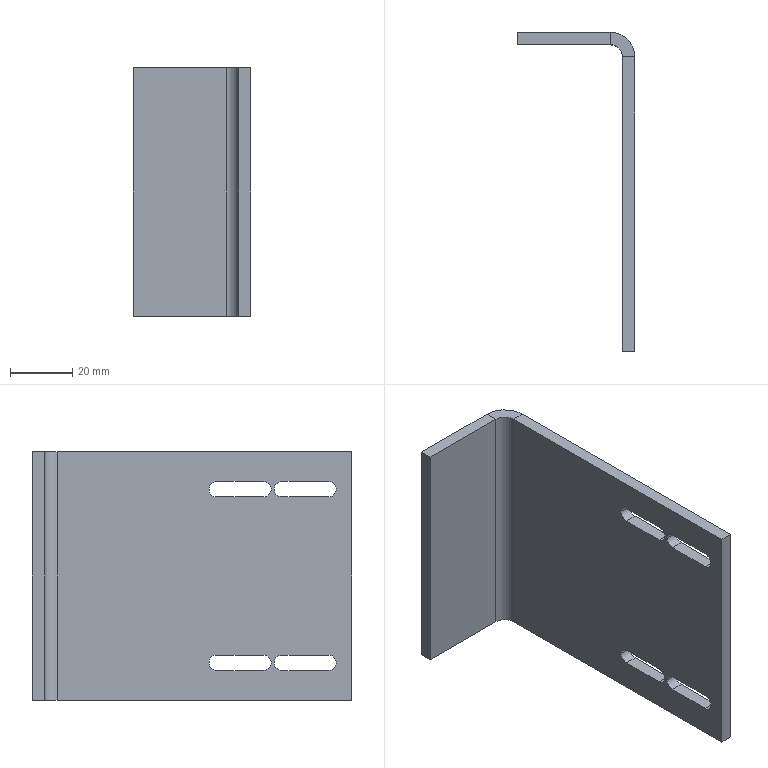Part | STEP file | 13-Positioning switch bracket | 1 solid | 34 faces | box 38 x 103 x 80 mm | volume 41502 mm3 | plane 20 | cylinder 14 | commonest cylinder face diameters 5 x12 8 x1 16 x1